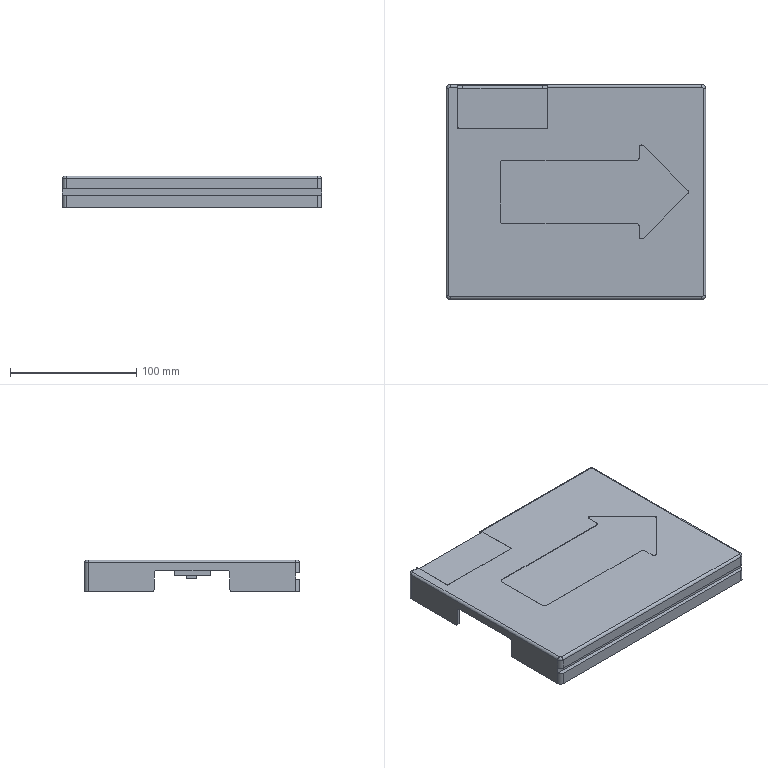NC program | NX | posted with a generic post | part box 205 x 170 x 25 mm
Whole program:
N10 G17 G21 G94 G90
(DRILLING_COPY_1 , TOOL : D6A45)
N12 T01 M6
N14 G54
N16 G17 G0 G90 X100.5 Y-12. B0. C0. S5000 M3
N18 G43 Z30. H1
N20 G94 G81 G98 Z-0.6 F250. R3.
N22 X127.5 Y-19.5
N24 X193.5
N26 G80
N28 G0 X193.5 Y-19.5 Z30.
N30 M5
(DRILLING_COPY_COPY , TOOL : 2.5ZT)
N32 T22 M6
N34 G54
N36 G17 G0 G90 X100.5 Y-12. B0. C0. S1447 M3
N38 G43 Z30. H22
N40 G94 G83 G98 Z-7.251 F100. Q2. R3.
N42 X127.5 Y-19.5
N44 X193.5
N46 G80
N48 G0 X193.5 Y-19.5 Z30.
N50 M5
(FLOOR_WALL_1_COPY_COPY , TOOL : D4)
N52 T17 M6
N54 G54
N56 G17 G0 G90 X174.118 Y-10.4 B0. C0. S9500 M3
N58 G43 Z30. H17
N60 Z1.5
N62 G94 G1 X184.4 Z0.961 F1000.
N64 Y-9.6 Z0.919
N66 X160.5 Z-0.333
N68 X136.6 F1450.
N70 Y-10.4
N72 X184.4
N74 Y-9.6
N76 X160.5
N78 Y-7.2
N80 X134.2
N82 Y-12.8
N84 X186.8
N86 Y-7.2
N88 X160.5
N90 Y-4.8
N92 X131.8
N94 Y-15.2
N96 X189.2
N98 Y-4.8
N100 X160.5
N102 Y-2.4
N104 X129.4
N106 Y-17.6
N108 X191.6
N110 Y-2.4
N112 X160.5
N114 Y0.
N116 X127.
N118 Y-20.
N120 X194.
N122 Y0.
N124 X160.5
N126 Z1.167
N128 G0 X174.118 Y-10.4
N130 G1 X184.4 Z0.628 F1000.
N132 Y-9.6 Z0.586
N134 X160.5 Z-0.667
N136 X136.6 F1450.
N138 Y-10.4
N140 X184.4
N142 Y-9.6
N144 X160.5
N146 Y-7.2
N148 X134.2
N150 Y-12.8
N152 X186.8
N154 Y-7.2
N156 X160.5
N158 Y-4.8
N160 X131.8
N162 Y-15.2
N164 X189.2
N166 Y-4.8
N168 X160.5
N170 Y-2.4
N172 X129.4
N174 Y-17.6
N176 X191.6
N178 Y-2.4
N180 X160.5
N182 Y0.
N184 X127.
N186 Y-20.
N188 X194.
N190 Y0.
N192 X160.5
N194 Z0.833
N196 G0 X174.118 Y-10.4
N198 G1 X184.4 Z0.294 F1000.
N200 Y-9.6 Z0.253
N202 X160.5 Z-1.
N204 X136.6 F1450.
N206 Y-10.4
N208 X184.4
N210 Y-9.6
N212 X160.5
N214 Y-7.2
N216 X134.2
N218 Y-12.8
N220 X186.8
N222 Y-7.2
N224 X160.5
N226 Y-4.8
N228 X131.8
N230 Y-15.2
N232 X189.2
N234 Y-4.8
N236 X160.5
N238 Y-2.4
N240 X129.4
N242 Y-17.6
N244 X191.6
N246 Y-2.4
N248 X160.5
N250 Y0.
N252 X127.
N254 Y-20.
N256 X194.
N258 Y0.
N260 X160.5
N262 Z0.5
N264 G0 Z30.
(ZLEVEL_PROFILE_COPY , TOOL : D4)
N266 X131.713 Y1.579
N268 Z1.609
N270 G1 Z-1.391 F1000.
N272 X131.198 Y1.281
N274 G3 X130.998 Y0.935 R0.4
N276 G1 X131. Y-0.814
N278 Y-1.008
N280 Y-15.992
N282 X131.039 Y-16.
N284 X189.985
N286 X190. Y-15.97
N288 Y-1.015
N290 X190.002 Y-1.
N292 X190. Y0.926
N294 X190.002 Y0.935
N296 G3 X189.801 Y1.281 R0.4
N298 G1 X189.287 Y1.578
N300 Z1.609
N302 G0 X189.283 Y1.685 Z1.217
N304 G1 Z-1.783
N306 X189.8 Y1.387
N308 G2 X190. Y1.04 R0.4
N310 G1 X190.002 Y-1.
N312 X190. Y-1.015
N314 Y-15.97
N316 X189.984 Y-16.
N318 X131.039
N320 X131. Y-15.992
N322 Y-0.818
N324 X130.998 Y-0.797
N326 X131. Y1.04
N328 G2 X131.2 Y1.387 R0.4
N330 G1 X131.717 Y1.685
N332 Z1.217
N334 G0 X131.714 Y1.807 Z0.826
N336 G1 Z-2.174
N338 X131.2 Y1.51
N340 G3 X130.999 Y1.163 R0.4
N342 G1 X130.998 Y-0.797
N344 X131. Y-0.818
N346 Y-15.992
N348 X131.039 Y-16.
N350 X189.984
N352 X190. Y-15.97
N354 Y-1.015
N356 X190.002 Y-1.
N358 X190.001 Y1.163
N360 G3 X189.8 Y1.51 R0.4
N362 G1 X189.286 Y1.807
N364 Z0.826
N366 G0 X189.279 Y1.837 Z0.435
N368 G1 Z-2.565
N370 X189.8 Y1.536
N372 G2 X190. Y1.19 R0.4
N374 G1 X190.002 Y-1.
N376 X190. Y-1.015
N378 Y-15.97
N380 X189.983 Y-16.
N382 X131.039
N384 X131. Y-15.992
N386 Y-0.818
N388 X130.998 Y-0.797
N390 X131. Y1.19
N392 G2 X131.2 Y1.536 R0.4
N394 G1 X131.721 Y1.837
N396 Z0.435
N398 G0 X131.725 Y1.839 Z0.043
N400 G1 Z-2.957
N402 X131.2 Y1.536
N404 G3 X131. Y1.19 R0.4
N406 G1 X130.998 Y-0.797
N408 X131. Y-0.818
N410 Y-15.992
N412 X131.039 Y-16.
N414 X189.982
N416 X190. Y-15.97
N418 Y-1.001
N420 X190.002 Y-0.779
N422 X190. Y1.19
N424 G3 X189.8 Y1.536 R0.4
N426 G1 X189.275 Y1.839
N428 Z0.043
N430 G0 Z-0.348
N432 G1 Z-3.348
N434 X189.8 Y1.536
N436 G2 X190. Y1.19 R0.4
N438 G1 X190.002 Y-0.691
N440 X190. Y-1.
N442 Y-15.97
N444 X189.981 Y-16.
N446 X131.039
N448 X131. Y-15.992
N450 Y-1.
N452 X130.998 Y-0.797
N454 X131. Y1.19
N456 G2 X131.2 Y1.536 R0.4
N458 G1 X131.725 Y1.839
N460 Z-0.348
N462 G0 X131.726 Z-0.739
N464 G1 Z-3.739
N466 X131.2 Y1.536
N468 G3 X131. Y1.19 R0.4
N470 G1 X130.998 Y-0.797
N472 X131. Y-1.
N474 Y-15.992
N476 X131.039 Y-16.
N478 X189.98
N480 X190. Y-15.97
N482 Y-1.
N484 X190.002 Y-0.691
N486 X190. Y1.19
N488 G3 X189.8 Y1.536 R0.4
N490 G1 X189.275 Y1.839
N492 Z-0.739
N494 G0 Z-1.13
N496 G1 Z-4.13
N498 X189.8 Y1.536
N500 G2 X190. Y1.19 R0.4
N502 G1 X190.002 Y-0.691
N504 X190. Y-1.
N506 Y-15.97
N508 X189.978 Y-16.
N510 X131.039
N512 X131. Y-15.992
N514 Y-1.
N516 X130.999 Y-0.797
N518 X131. Y1.19
N520 G2 X131.2 Y1.536 R0.4
N522 G1 X131.726 Y1.839
N524 Z-1.13
N526 G0 Z-1.522
N528 G1 Z-4.522
N530 X131.2 Y1.536
N532 G3 X131. Y1.19 R0.4
N534 G1 X130.999 Y-0.797
N536 X131. Y-1.
N538 Y-15.992
N540 X131.039 Y-16.
N542 X189.99
N544 X190. Y-15.953
N546 Y-1.
N548 X190.001 Y-0.691
N550 X190. Y1.19
N552 G3 X189.8 Y1.536 R0.4
N554 G1 X189.275 Y1.839
N556 Z-1.522
N558 G0 Z-1.913
N560 G1 Z-4.913
N562 X189.8 Y1.536
N564 G2 X190. Y1.19 R0.4
N566 G1 X190.001 Y-0.691
N568 X190. Y-1.
N570 Y-15.953
N572 X189.99 Y-16.
N574 X131.039
N576 X131. Y-15.992
N578 Y-1.
N580 X130.999 Y-0.797
N582 X131. Y1.19
N584 G2 X131.2 Y1.536 R0.4
N586 G1 X131.726 Y1.839
N588 Z-1.913
N590 G0 Z-2.304
N592 G1 Z-5.304
N594 X131.2 Y1.536
N596 G3 X131. Y1.19 R0.4
N598 G1 X130.999 Y-0.797
N600 X131. Y-1.
N602 Y-15.992
N604 X131.042 Y-16.
N606 X189.99
N608 X190. Y-15.953
N610 Y-1.
N612 X190.001 Y-0.691
N614 X190. Y1.19
N616 G3 X189.8 Y1.536 R0.4
N618 G1 X189.275 Y1.839
N620 Z-2.304
N622 G0 Z-2.696
N624 G1 Z-5.696
N626 X189.8 Y1.536
N628 G2 X190. Y1.19 R0.4
N630 G1 X190.001 Y-0.691
N632 X190. Y-1.
N634 Y-15.953
N636 X189.99 Y-16.
N638 X131.042
N640 X131. Y-15.992
N642 Y-1.
N644 X130.999 Y-0.797
N646 X131. Y1.19
N648 G2 X131.2 Y1.536 R0.4
N650 G1 X131.726 Y1.839
N652 Z-2.696
N654 G0 Z-3.087
N656 G1 Z-6.087
N658 X131.2 Y1.536
N660 G3 X131. Y1.19 R0.4
N662 G1 X130.999 Y-0.797
N664 X131. Y-1.
N666 Y-15.992
N668 X131.042 Y-16.
N670 X189.99
N672 X190. Y-15.953
N674 Y-1.
N676 X190.001 Y-0.691
N678 X190. Y1.19
N680 G3 X189.8 Y1.536 R0.4
N682 G1 X189.275 Y1.839
N684 Z-3.087
N686 G0 Z-3.478
N688 G1 Z-6.478
N690 X189.8 Y1.536
N692 G2 X190. Y1.19 R0.4
N694 G1 X190.001 Y-0.691
N696 X190. Y-1.
N698 Y-15.953
N700 X189.99 Y-16.
N702 X131.042
N704 X131. Y-15.992
N706 Y-1.
N708 X130.999 Y-0.797
N710 X131. Y1.19
N712 G2 X131.2 Y1.536 R0.4
N714 G1 X131.726 Y1.839
N716 Z-3.478
N718 G0 Z-3.87
N720 G1 Z-6.87
N722 X131.2 Y1.536
N724 G3 X131. Y1.19 R0.4
N726 G1 X130.999 Y-0.797
N728 X131. Y-1.
N730 Y-15.992
N732 X131.042 Y-16.
N734 X189.99
N736 X190. Y-15.953
N738 Y-1.
N740 X190.001 Y-0.691
N742 X190. Y1.19
N744 G3 X189.8 Y1.536 R0.4
N746 G1 X189.275 Y1.839
N748 Z-3.87
N750 G0 Z-4.261
N752 G1 Z-7.261
N754 X189.8 Y1.536
N756 G2 X190. Y1.19 R0.4
N758 G1 X190.001 Y-0.691
N760 X190. Y-1.
N762 Y-15.953
N764 X189.99 Y-16.
N766 X131.042
N768 X131. Y-15.992
N770 Y-1.
N772 X130.999 Y-0.797
N774 X131. Y1.19
N776 G2 X131.2 Y1.536 R0.4
N778 G1 X131.726 Y1.839
N780 Z-4.261
N782 G0 Z-4.652
N784 G1 Z-7.652
N786 X131.2 Y1.536
N788 G3 X131. Y1.19 R0.4
N790 G1 X130.999 Y-0.797
N792 X131. Y-1.
N794 Y-15.992
N796 X131.042 Y-16.
N798 X189.99
N800 X190. Y-15.953
N802 Y-1.
N804 X190.001 Y-0.691
N806 X190. Y1.19
N808 G3 X189.8 Y1.536 R0.4
N810 G1 X189.275 Y1.839
N812 Z-4.652
N814 G0 Z-5.043
N816 G1 Z-8.043
N818 X189.8 Y1.536
N820 G2 X190. Y1.19 R0.4
N822 G1 X190.001 Y-0.691
N824 X190. Y-1.
N826 Y-15.953
N828 X189.99 Y-16.
N830 X131.042
N832 X131. Y-15.992
N834 Y-1.
N836 X130.999 Y-0.797
N838 X131. Y1.19
N840 G2 X131.2 Y1.536 R0.4
N842 G1 X131.728 Y1.84
N844 Z-5.043
N846 G0 Z-5.435
N848 G1 Z-8.435
N850 X131.2 Y1.536
N852 G3 X131. Y1.19 R0.4
N854 G1 X130.999 Y-0.797
N856 X131. Y-1.
N858 Y-15.992
N860 X131.042 Y-16.
N862 X189.99
N864 X190. Y-15.953
N866 Y-1.
N868 X190.001 Y-0.691
N870 X190. Y1.19
N872 G3 X189.8 Y1.536 R0.4
N874 G1 X189.275 Y1.839
N876 Z-5.435
N878 G0 X189.274 Z-5.826
N880 G1 Z-8.826
N882 X189.8 Y1.536
N884 G2 X190. Y1.19 R0.4
N886 G1 X190.001 Y-0.691
N888 X190. Y-1.
N890 Y-15.953
N892 X189.99 Y-16.
N894 X131.042
N896 X131. Y-15.992
N898 Y-1.
N900 X130.999 Y-0.797
N902 X131. Y1.19
N904 G2 X131.2 Y1.536 R0.4
N906 G1 X131.728 Y1.84
N908 Z-5.826
N910 G0 Z-6.217
N912 G1 Z-9.217
N914 X131.2 Y1.536
N916 G3 X131. Y1.19 R0.4
N918 G1 X130.999 Y-0.797
N920 X131. Y-1.
N922 Y-15.992
N924 X131.042 Y-16.
N926 X189.99
N928 X190. Y-15.953
N930 Y-1.
N932 X190.001 Y-0.691
N934 X190. Y1.19
N936 G3 X189.8 Y1.536 R0.4
N938 G1 X189.274 Y1.839
N940 Z-6.217
N942 G0 Z-6.609
N944 G1 Z-9.609
N946 X189.8 Y1.536
N948 G2 X190. Y1.19 R0.4
N950 G1 X190.001 Y-0.691
N952 X190. Y-1.
N954 Y-15.953
N956 X189.99 Y-16.
N958 X131.042
N960 X131. Y-15.992
N962 Y-1.
N964 X130.999 Y-0.797
N966 X131. Y1.19
N968 G2 X131.2 Y1.536 R0.4
N970 G1 X131.728 Y1.84
N972 Z-6.609
N974 G0 X131.727 Y1.841 Z-7.
N976 G1 Z-10.
N978 X131.2 Y1.536
N980 G3 X131. Y1.19 R0.4
N982 G1 Y-1.
N984 Y-15.992
N986 X131.042 Y-16.
N988 X189.99
N990 X190. Y-15.953
N992 Y-1.
N994 X190.001 Y-0.691
N996 X190. Y1.19
N998 G3 X189.8 Y1.536 R0.4
N1000 G1 X189.274 Y1.839
N1002 Z-7.
N1004 G0 Z30.
N1006 M5
N1008 M2